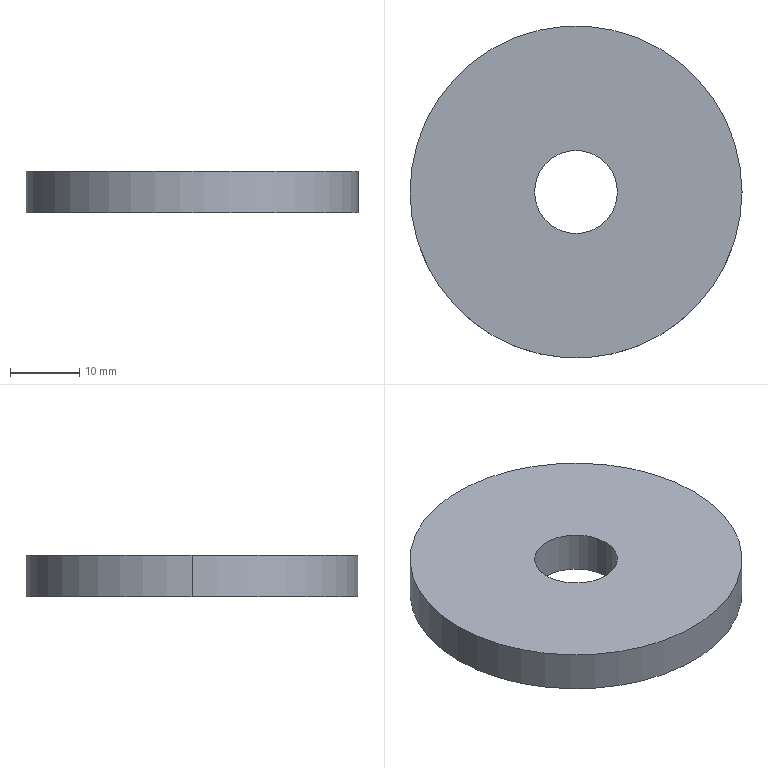Part | STEP file | HXGR200008-05-12-02 | 1 solid | 6 faces | box 48 x 48 x 6 mm | volume 10179 mm3 | cylinder 4 | plane 2 | commonest cylinder face diameters 12 x2 48 x2
STEP:
#1=CARTESIAN_POINT('',(-6.,0.,6.));
#2=VERTEX_POINT('',#1);
#3=CARTESIAN_POINT('',(6.,0.,6.));
#4=VERTEX_POINT('',#3);
#5=CARTESIAN_POINT('',(0.,0.,6.));
#6=DIRECTION('',(0.,0.,1.));
#7=DIRECTION('',(1.,0.,0.));
#8=AXIS2_PLACEMENT_3D('',#5,#6,#7);
#9=CIRCLE('',#8,6.);
#10=EDGE_CURVE('',#2,#4,#9,.T.);
#11=ORIENTED_EDGE('',*,*,#10,.T.);
#12=CARTESIAN_POINT('',(6.,0.,0.));
#13=VERTEX_POINT('',#12);
#14=CARTESIAN_POINT('',(6.,0.,6.));
#15=DIRECTION('',(0.,0.,-1.));
#16=VECTOR('',#15,1000.);
#17=LINE('',#14,#16);
#18=EDGE_CURVE('',#4,#13,#17,.T.);
#19=ORIENTED_EDGE('',*,*,#18,.T.);
#20=CARTESIAN_POINT('',(-6.,0.,0.));
#21=VERTEX_POINT('',#20);
#22=CARTESIAN_POINT('',(0.,0.,0.));
#23=DIRECTION('',(0.,0.,1.));
#24=DIRECTION('',(1.,0.,0.));
#25=AXIS2_PLACEMENT_3D('',#22,#23,#24);
#26=CIRCLE('',#25,6.);
#27=EDGE_CURVE('',#21,#13,#26,.T.);
#28=ORIENTED_EDGE('',*,*,#27,.F.);
#29=CARTESIAN_POINT('',(-6.,0.,6.));
#30=DIRECTION('',(0.,0.,-1.));
#31=VECTOR('',#30,1000.);
#32=LINE('',#29,#31);
#33=EDGE_CURVE('',#2,#21,#32,.T.);
#34=ORIENTED_EDGE('',*,*,#33,.F.);
#35=EDGE_LOOP('',(#11,#19,#28,#34));
#36=FACE_OUTER_BOUND('',#35,.T.);
#37=CARTESIAN_POINT('',(0.,0.,6.));
#38=DIRECTION('',(0.,0.,-1.));
#39=DIRECTION('',(-1.,0.,0.));
#40=AXIS2_PLACEMENT_3D('',#37,#38,#39);
#41=CYLINDRICAL_SURFACE('',#40,6.);
#42=ADVANCED_FACE('',(#36),#41,.F.);
#43=CARTESIAN_POINT('',(24.,0.,6.));
#44=VERTEX_POINT('',#43);
#45=CARTESIAN_POINT('',(-24.,0.,6.));
#46=VERTEX_POINT('',#45);
#47=CARTESIAN_POINT('',(0.,0.,6.));
#48=DIRECTION('',(0.,0.,1.));
#49=DIRECTION('',(1.,0.,0.));
#50=AXIS2_PLACEMENT_3D('',#47,#48,#49);
#51=CIRCLE('',#50,24.);
#52=EDGE_CURVE('',#44,#46,#51,.T.);
#53=ORIENTED_EDGE('',*,*,#52,.F.);
#54=CARTESIAN_POINT('',(24.,0.,0.));
#55=VERTEX_POINT('',#54);
#56=CARTESIAN_POINT('',(24.,0.,6.));
#57=DIRECTION('',(0.,0.,-1.));
#58=VECTOR('',#57,1000.);
#59=LINE('',#56,#58);
#60=EDGE_CURVE('',#44,#55,#59,.T.);
#61=ORIENTED_EDGE('',*,*,#60,.T.);
#62=CARTESIAN_POINT('',(-24.,0.,0.));
#63=VERTEX_POINT('',#62);
#64=CARTESIAN_POINT('',(0.,0.,0.));
#65=DIRECTION('',(0.,0.,1.));
#66=DIRECTION('',(1.,0.,0.));
#67=AXIS2_PLACEMENT_3D('',#64,#65,#66);
#68=CIRCLE('',#67,24.);
#69=EDGE_CURVE('',#55,#63,#68,.T.);
#70=ORIENTED_EDGE('',*,*,#69,.T.);
#71=CARTESIAN_POINT('',(-24.,0.,6.));
#72=DIRECTION('',(0.,0.,-1.));
#73=VECTOR('',#72,1000.);
#74=LINE('',#71,#73);
#75=EDGE_CURVE('',#46,#63,#74,.T.);
#76=ORIENTED_EDGE('',*,*,#75,.F.);
#77=EDGE_LOOP('',(#53,#61,#70,#76));
#78=FACE_OUTER_BOUND('',#77,.T.);
#79=CARTESIAN_POINT('',(0.,0.,6.));
#80=DIRECTION('',(0.,0.,-1.));
#81=DIRECTION('',(-1.,0.,0.));
#82=AXIS2_PLACEMENT_3D('',#79,#80,#81);
#83=CYLINDRICAL_SURFACE('',#82,24.);
#84=ADVANCED_FACE('',(#78),#83,.T.);
#85=CARTESIAN_POINT('',(0.,0.,6.));
#86=DIRECTION('',(0.,0.,1.));
#87=DIRECTION('',(1.,0.,0.));
#88=AXIS2_PLACEMENT_3D('',#85,#86,#87);
#89=CIRCLE('',#88,24.);
#90=EDGE_CURVE('',#46,#44,#89,.T.);
#91=ORIENTED_EDGE('',*,*,#90,.T.);
#92=ORIENTED_EDGE('',*,*,#52,.T.);
#93=EDGE_LOOP('',(#91,#92));
#94=FACE_OUTER_BOUND('',#93,.T.);
#95=ORIENTED_EDGE('',*,*,#10,.F.);
#96=CARTESIAN_POINT('',(0.,0.,6.));
#97=DIRECTION('',(0.,0.,1.));
#98=DIRECTION('',(1.,0.,0.));
#99=AXIS2_PLACEMENT_3D('',#96,#97,#98);
#100=CIRCLE('',#99,6.);
#101=EDGE_CURVE('',#4,#2,#100,.T.);
#102=ORIENTED_EDGE('',*,*,#101,.F.);
#103=EDGE_LOOP('',(#95,#102));
#104=FACE_BOUND('',#103,.T.);
#105=CARTESIAN_POINT('',(0.,0.,6.));
#106=DIRECTION('',(0.,0.,1.));
#107=DIRECTION('',(1.,0.,0.));
#108=AXIS2_PLACEMENT_3D('',#105,#106,#107);
#109=PLANE('',#108);
#110=ADVANCED_FACE('',(#94,#104),#109,.T.);
#111=CARTESIAN_POINT('',(0.,0.,0.));
#112=DIRECTION('',(0.,0.,1.));
#113=DIRECTION('',(1.,0.,0.));
#114=AXIS2_PLACEMENT_3D('',#111,#112,#113);
#115=CIRCLE('',#114,24.);
#116=EDGE_CURVE('',#63,#55,#115,.T.);
#117=ORIENTED_EDGE('',*,*,#116,.F.);
#118=ORIENTED_EDGE('',*,*,#69,.F.);
#119=EDGE_LOOP('',(#117,#118));
#120=FACE_OUTER_BOUND('',#119,.T.);
#121=ORIENTED_EDGE('',*,*,#27,.T.);
#122=CARTESIAN_POINT('',(0.,0.,0.));
#123=DIRECTION('',(0.,0.,1.));
#124=DIRECTION('',(1.,0.,0.));
#125=AXIS2_PLACEMENT_3D('',#122,#123,#124);
#126=CIRCLE('',#125,6.);
#127=EDGE_CURVE('',#13,#21,#126,.T.);
#128=ORIENTED_EDGE('',*,*,#127,.T.);
#129=EDGE_LOOP('',(#121,#128));
#130=FACE_BOUND('',#129,.T.);
#131=CARTESIAN_POINT('',(0.,0.,0.));
#132=DIRECTION('',(0.,0.,1.));
#133=DIRECTION('',(1.,0.,0.));
#134=AXIS2_PLACEMENT_3D('',#131,#132,#133);
#135=PLANE('',#134);
#136=ADVANCED_FACE('',(#120,#130),#135,.F.);
#137=ORIENTED_EDGE('',*,*,#60,.F.);
#138=ORIENTED_EDGE('',*,*,#90,.F.);
#139=ORIENTED_EDGE('',*,*,#75,.T.);
#140=ORIENTED_EDGE('',*,*,#116,.T.);
#141=EDGE_LOOP('',(#137,#138,#139,#140));
#142=FACE_OUTER_BOUND('',#141,.T.);
#143=CARTESIAN_POINT('',(0.,0.,6.));
#144=DIRECTION('',(0.,0.,-1.));
#145=DIRECTION('',(-1.,0.,0.));
#146=AXIS2_PLACEMENT_3D('',#143,#144,#145);
#147=CYLINDRICAL_SURFACE('',#146,24.);
#148=ADVANCED_FACE('',(#142),#147,.T.);
#149=ORIENTED_EDGE('',*,*,#18,.F.);
#150=ORIENTED_EDGE('',*,*,#101,.T.);
#151=ORIENTED_EDGE('',*,*,#33,.T.);
#152=ORIENTED_EDGE('',*,*,#127,.F.);
#153=EDGE_LOOP('',(#149,#150,#151,#152));
#154=FACE_OUTER_BOUND('',#153,.T.);
#155=CARTESIAN_POINT('',(0.,0.,6.));
#156=DIRECTION('',(0.,0.,-1.));
#157=DIRECTION('',(-1.,0.,0.));
#158=AXIS2_PLACEMENT_3D('',#155,#156,#157);
#159=CYLINDRICAL_SURFACE('',#158,6.);
#160=ADVANCED_FACE('',(#154),#159,.F.);
#161=CLOSED_SHELL('',(#42,#84,#110,#136,#148,#160));
#162=MANIFOLD_SOLID_BREP('',#161);
#163=CARTESIAN_POINT('',(0.,0.,0.));
#164=DIRECTION('',(0.,0.,1.));
#165=DIRECTION('',(1.,0.,0.));
#166=AXIS2_PLACEMENT_3D('',#163,#164,#165);
#167=(LENGTH_UNIT()NAMED_UNIT(*)SI_UNIT(.MILLI.,.METRE.));
#168=UNCERTAINTY_MEASURE_WITH_UNIT(LENGTH_MEASURE(0.00001),#167,'','');
#169=(NAMED_UNIT(*)PLANE_ANGLE_UNIT()SI_UNIT($,.RADIAN.));
#170=(NAMED_UNIT(*)SI_UNIT($,.STERADIAN.)SOLID_ANGLE_UNIT());
#171=(GEOMETRIC_REPRESENTATION_CONTEXT(3)GLOBAL_UNCERTAINTY_ASSIGNED_CONTEXT((#168))GLOBAL_UNIT_ASSIGNED_CONTEXT((#167,#169,#170))REPRESENTATION_CONTEXT('',''));
#172=ADVANCED_BREP_SHAPE_REPRESENTATION('',(#162,#166),#171);